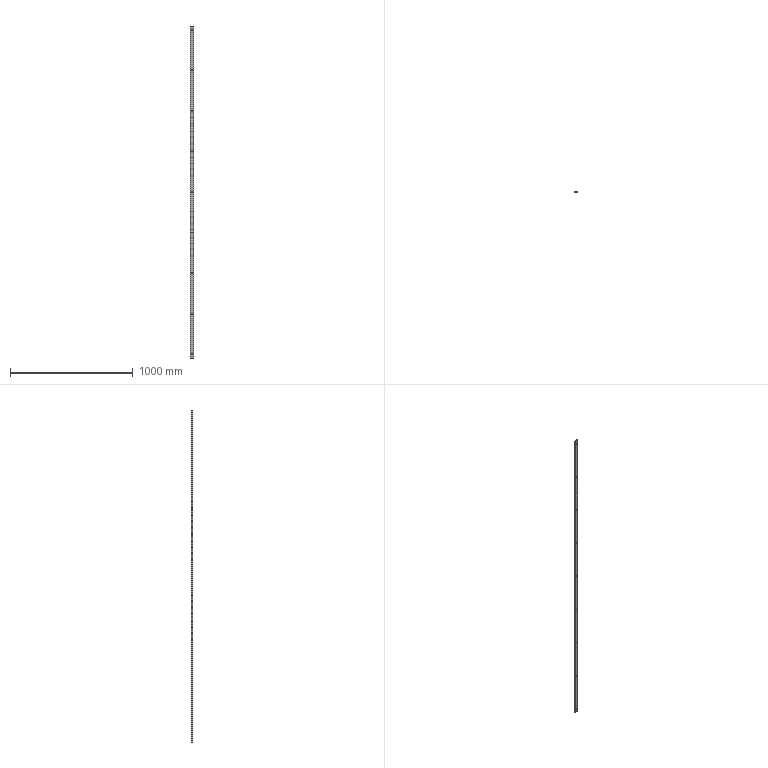Part | STEP file | PE_01 | 1 solid | 25 faces | box 31 x 10 x 2700 mm | volume 827532 mm3 | cone 9 | cylinder 9 | plane 7 | commonest cylinder face diameters 6.5 x9